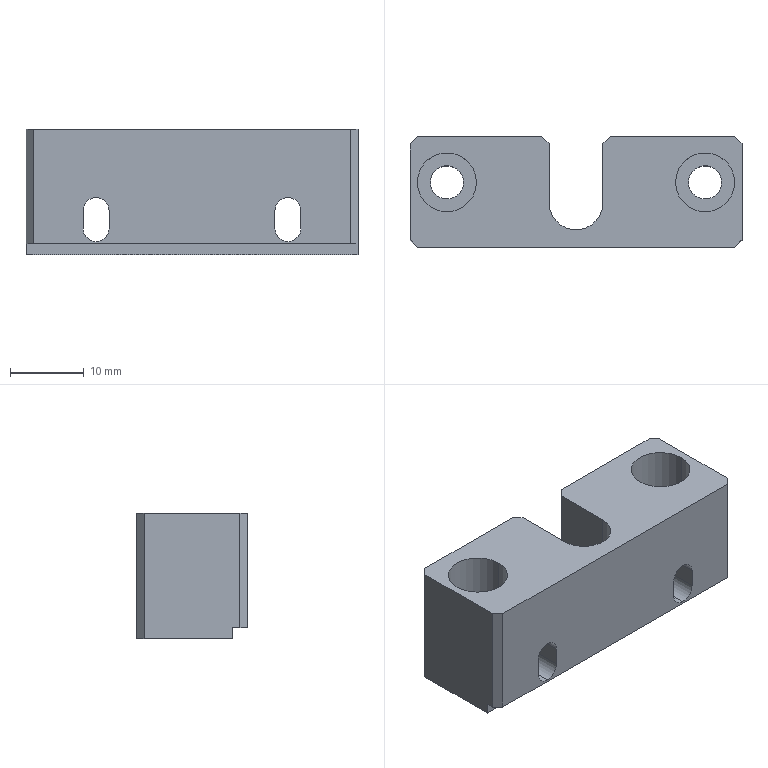Part | SolidWorks | features BaseBody 1 | 1 solid | 46 faces | box 45 x 15 x 17 mm | volume 8178 mm3 | plane 23 | cylinder 19 | cone 4 | commonest cylinder face diameters 3.5 x6 4 x4 4.5 x4 8 x4 7.3 x1
STEP:
#1=CARTESIAN_POINT('',(35.5,15.,-2.25));
#2=VERTEX_POINT('',#1);
#3=CARTESIAN_POINT('',(37.25,15.,-0.5));
#4=VERTEX_POINT('',#3);
#5=CARTESIAN_POINT('',(35.5,15.,-0.5));
#6=DIRECTION('',(0.,-1.,0.));
#7=DIRECTION('',(0.,0.,-1.));
#8=AXIS2_PLACEMENT_3D('',#5,#6,#7);
#9=CIRCLE('',#8,1.75);
#10=EDGE_CURVE('',#2,#4,#9,.T.);
#11=ORIENTED_EDGE('',*,*,#10,.F.);
#12=CARTESIAN_POINT('',(35.5,0.,-2.25));
#13=VERTEX_POINT('',#12);
#14=CARTESIAN_POINT('',(35.5,15.,-2.25));
#15=DIRECTION('',(0.,-1.,0.));
#16=VECTOR('',#15,1000.);
#17=LINE('',#14,#16);
#18=EDGE_CURVE('',#2,#13,#17,.T.);
#19=ORIENTED_EDGE('',*,*,#18,.T.);
#20=CARTESIAN_POINT('',(37.25,0.,-0.5));
#21=VERTEX_POINT('',#20);
#22=CARTESIAN_POINT('',(35.5,0.,-0.5));
#23=DIRECTION('',(0.,1.,0.));
#24=DIRECTION('',(0.,0.,-1.));
#25=AXIS2_PLACEMENT_3D('',#22,#23,#24);
#26=CIRCLE('',#25,1.75);
#27=EDGE_CURVE('',#21,#13,#26,.T.);
#28=ORIENTED_EDGE('',*,*,#27,.F.);
#29=CARTESIAN_POINT('',(37.25,15.,-0.5));
#30=DIRECTION('',(0.,-1.,0.));
#31=VECTOR('',#30,1000.);
#32=LINE('',#29,#31);
#33=EDGE_CURVE('',#4,#21,#32,.T.);
#34=ORIENTED_EDGE('',*,*,#33,.F.);
#35=EDGE_LOOP('',(#11,#19,#28,#34));
#36=FACE_OUTER_BOUND('',#35,.T.);
#37=CARTESIAN_POINT('',(35.5,15.,-0.5));
#38=DIRECTION('',(0.,-1.,0.));
#39=DIRECTION('',(0.,0.,-1.));
#40=AXIS2_PLACEMENT_3D('',#37,#38,#39);
#41=CYLINDRICAL_SURFACE('',#40,1.75);
#42=ADVANCED_FACE('',(#36),#41,.F.);
#43=CARTESIAN_POINT('',(9.5,15.,-2.25));
#44=VERTEX_POINT('',#43);
#45=CARTESIAN_POINT('',(11.25,15.,-0.5));
#46=VERTEX_POINT('',#45);
#47=CARTESIAN_POINT('',(9.5,15.,-0.5));
#48=DIRECTION('',(0.,-1.,0.));
#49=DIRECTION('',(0.,0.,-1.));
#50=AXIS2_PLACEMENT_3D('',#47,#48,#49);
#51=CIRCLE('',#50,1.75);
#52=EDGE_CURVE('',#44,#46,#51,.T.);
#53=ORIENTED_EDGE('',*,*,#52,.F.);
#54=CARTESIAN_POINT('',(9.5,0.,-2.25));
#55=VERTEX_POINT('',#54);
#56=CARTESIAN_POINT('',(9.5,15.,-2.25));
#57=DIRECTION('',(0.,-1.,0.));
#58=VECTOR('',#57,1000.);
#59=LINE('',#56,#58);
#60=EDGE_CURVE('',#44,#55,#59,.T.);
#61=ORIENTED_EDGE('',*,*,#60,.T.);
#62=CARTESIAN_POINT('',(11.25,0.,-0.5));
#63=VERTEX_POINT('',#62);
#64=CARTESIAN_POINT('',(9.5,0.,-0.5));
#65=DIRECTION('',(0.,1.,0.));
#66=DIRECTION('',(0.,0.,-1.));
#67=AXIS2_PLACEMENT_3D('',#64,#65,#66);
#68=CIRCLE('',#67,1.75);
#69=EDGE_CURVE('',#63,#55,#68,.T.);
#70=ORIENTED_EDGE('',*,*,#69,.F.);
#71=CARTESIAN_POINT('',(11.25,15.,-0.5));
#72=DIRECTION('',(0.,-1.,0.));
#73=VECTOR('',#72,1000.);
#74=LINE('',#71,#73);
#75=EDGE_CURVE('',#46,#63,#74,.T.);
#76=ORIENTED_EDGE('',*,*,#75,.F.);
#77=EDGE_LOOP('',(#53,#61,#70,#76));
#78=FACE_OUTER_BOUND('',#77,.T.);
#79=CARTESIAN_POINT('',(9.5,15.,-0.5));
#80=DIRECTION('',(0.,-1.,0.));
#81=DIRECTION('',(0.,0.,-1.));
#82=AXIS2_PLACEMENT_3D('',#79,#80,#81);
#83=CYLINDRICAL_SURFACE('',#82,1.75);
#84=ADVANCED_FACE('',(#78),#83,.F.);
#85=CARTESIAN_POINT('',(36.,8.8,7.));
#86=VERTEX_POINT('',#85);
#87=CARTESIAN_POINT('',(44.,8.8,7.));
#88=VERTEX_POINT('',#87);
#89=CARTESIAN_POINT('',(40.,8.8,7.));
#90=DIRECTION('',(0.,0.,1.));
#91=DIRECTION('',(1.,0.,0.));
#92=AXIS2_PLACEMENT_3D('',#89,#90,#91);
#93=CIRCLE('',#92,4.);
#94=EDGE_CURVE('',#86,#88,#93,.T.);
#95=ORIENTED_EDGE('',*,*,#94,.F.);
#96=CARTESIAN_POINT('',(36.,8.8,13.));
#97=VERTEX_POINT('',#96);
#98=CARTESIAN_POINT('',(36.,8.8,13.));
#99=DIRECTION('',(0.,0.,1.));
#100=VECTOR('',#99,1000.);
#101=LINE('',#98,#100);
#102=EDGE_CURVE('',#86,#97,#101,.T.);
#103=ORIENTED_EDGE('',*,*,#102,.T.);
#104=CARTESIAN_POINT('',(44.,8.8,13.));
#105=VERTEX_POINT('',#104);
#106=CARTESIAN_POINT('',(40.,8.8,13.));
#107=DIRECTION('',(0.,0.,-1.));
#108=DIRECTION('',(1.,0.,0.));
#109=AXIS2_PLACEMENT_3D('',#106,#107,#108);
#110=CIRCLE('',#109,4.);
#111=EDGE_CURVE('',#105,#97,#110,.T.);
#112=ORIENTED_EDGE('',*,*,#111,.F.);
#113=CARTESIAN_POINT('',(44.,8.8,13.));
#114=DIRECTION('',(0.,0.,1.));
#115=VECTOR('',#114,1000.);
#116=LINE('',#113,#115);
#117=EDGE_CURVE('',#88,#105,#116,.T.);
#118=ORIENTED_EDGE('',*,*,#117,.F.);
#119=EDGE_LOOP('',(#95,#103,#112,#118));
#120=FACE_OUTER_BOUND('',#119,.T.);
#121=CARTESIAN_POINT('',(40.,8.8,13.));
#122=DIRECTION('',(0.,0.,1.));
#123=DIRECTION('',(1.,0.,0.));
#124=AXIS2_PLACEMENT_3D('',#121,#122,#123);
#125=CYLINDRICAL_SURFACE('',#124,4.);
#126=ADVANCED_FACE('',(#120),#125,.F.);
#127=CARTESIAN_POINT('',(1.,8.8,7.));
#128=VERTEX_POINT('',#127);
#129=CARTESIAN_POINT('',(9.,8.8,7.));
#130=VERTEX_POINT('',#129);
#131=CARTESIAN_POINT('',(5.,8.8,7.));
#132=DIRECTION('',(0.,0.,1.));
#133=DIRECTION('',(1.,0.,0.));
#134=AXIS2_PLACEMENT_3D('',#131,#132,#133);
#135=CIRCLE('',#134,4.);
#136=EDGE_CURVE('',#128,#130,#135,.T.);
#137=ORIENTED_EDGE('',*,*,#136,.F.);
#138=CARTESIAN_POINT('',(1.,8.8,13.));
#139=VERTEX_POINT('',#138);
#140=CARTESIAN_POINT('',(1.,8.8,13.));
#141=DIRECTION('',(0.,0.,1.));
#142=VECTOR('',#141,1000.);
#143=LINE('',#140,#142);
#144=EDGE_CURVE('',#128,#139,#143,.T.);
#145=ORIENTED_EDGE('',*,*,#144,.T.);
#146=CARTESIAN_POINT('',(9.,8.8,13.));
#147=VERTEX_POINT('',#146);
#148=CARTESIAN_POINT('',(5.,8.8,13.));
#149=DIRECTION('',(0.,0.,-1.));
#150=DIRECTION('',(1.,0.,0.));
#151=AXIS2_PLACEMENT_3D('',#148,#149,#150);
#152=CIRCLE('',#151,4.);
#153=EDGE_CURVE('',#147,#139,#152,.T.);
#154=ORIENTED_EDGE('',*,*,#153,.F.);
#155=CARTESIAN_POINT('',(9.,8.8,13.));
#156=DIRECTION('',(0.,0.,1.));
#157=VECTOR('',#156,1000.);
#158=LINE('',#155,#157);
#159=EDGE_CURVE('',#130,#147,#158,.T.);
#160=ORIENTED_EDGE('',*,*,#159,.F.);
#161=EDGE_LOOP('',(#137,#145,#154,#160));
#162=FACE_OUTER_BOUND('',#161,.T.);
#163=CARTESIAN_POINT('',(5.,8.8,13.));
#164=DIRECTION('',(0.,0.,1.));
#165=DIRECTION('',(1.,0.,0.));
#166=AXIS2_PLACEMENT_3D('',#163,#164,#165);
#167=CYLINDRICAL_SURFACE('',#166,4.);
#168=ADVANCED_FACE('',(#162),#167,.F.);
#169=CARTESIAN_POINT('',(37.75,8.8,-4.));
#170=VERTEX_POINT('',#169);
#171=CARTESIAN_POINT('',(42.25,8.8,-4.));
#172=VERTEX_POINT('',#171);
#173=CARTESIAN_POINT('',(40.,8.8,-4.));
#174=DIRECTION('',(0.,0.,1.));
#175=DIRECTION('',(1.,0.,0.));
#176=AXIS2_PLACEMENT_3D('',#173,#174,#175);
#177=CIRCLE('',#176,2.25);
#178=EDGE_CURVE('',#170,#172,#177,.T.);
#179=ORIENTED_EDGE('',*,*,#178,.F.);
#180=CARTESIAN_POINT('',(37.75,8.8,7.));
#181=VERTEX_POINT('',#180);
#182=CARTESIAN_POINT('',(37.75,8.8,13.));
#183=DIRECTION('',(0.,0.,1.));
#184=VECTOR('',#183,1000.);
#185=LINE('',#182,#184);
#186=EDGE_CURVE('',#170,#181,#185,.T.);
#187=ORIENTED_EDGE('',*,*,#186,.T.);
#188=CARTESIAN_POINT('',(42.25,8.8,7.));
#189=VERTEX_POINT('',#188);
#190=CARTESIAN_POINT('',(40.,8.8,7.));
#191=DIRECTION('',(0.,0.,1.));
#192=DIRECTION('',(1.,0.,0.));
#193=AXIS2_PLACEMENT_3D('',#190,#191,#192);
#194=CIRCLE('',#193,2.25);
#195=EDGE_CURVE('',#181,#189,#194,.T.);
#196=ORIENTED_EDGE('',*,*,#195,.T.);
#197=CARTESIAN_POINT('',(42.25,8.8,13.));
#198=DIRECTION('',(0.,0.,1.));
#199=VECTOR('',#198,1000.);
#200=LINE('',#197,#199);
#201=EDGE_CURVE('',#172,#189,#200,.T.);
#202=ORIENTED_EDGE('',*,*,#201,.F.);
#203=EDGE_LOOP('',(#179,#187,#196,#202));
#204=FACE_OUTER_BOUND('',#203,.T.);
#205=CARTESIAN_POINT('',(40.,8.8,13.));
#206=DIRECTION('',(0.,0.,1.));
#207=DIRECTION('',(1.,0.,0.));
#208=AXIS2_PLACEMENT_3D('',#205,#206,#207);
#209=CYLINDRICAL_SURFACE('',#208,2.25);
#210=ADVANCED_FACE('',(#204),#209,.F.);
#211=CARTESIAN_POINT('',(2.75,8.8,-4.));
#212=VERTEX_POINT('',#211);
#213=CARTESIAN_POINT('',(7.25,8.8,-4.));
#214=VERTEX_POINT('',#213);
#215=CARTESIAN_POINT('',(5.,8.8,-4.));
#216=DIRECTION('',(0.,0.,1.));
#217=DIRECTION('',(1.,0.,0.));
#218=AXIS2_PLACEMENT_3D('',#215,#216,#217);
#219=CIRCLE('',#218,2.25);
#220=EDGE_CURVE('',#212,#214,#219,.T.);
#221=ORIENTED_EDGE('',*,*,#220,.F.);
#222=CARTESIAN_POINT('',(2.75,8.8,7.));
#223=VERTEX_POINT('',#222);
#224=CARTESIAN_POINT('',(2.75,8.8,13.));
#225=DIRECTION('',(0.,0.,1.));
#226=VECTOR('',#225,1000.);
#227=LINE('',#224,#226);
#228=EDGE_CURVE('',#212,#223,#227,.T.);
#229=ORIENTED_EDGE('',*,*,#228,.T.);
#230=CARTESIAN_POINT('',(7.25,8.8,7.));
#231=VERTEX_POINT('',#230);
#232=CARTESIAN_POINT('',(5.,8.8,7.));
#233=DIRECTION('',(0.,0.,1.));
#234=DIRECTION('',(1.,0.,0.));
#235=AXIS2_PLACEMENT_3D('',#232,#233,#234);
#236=CIRCLE('',#235,2.25);
#237=EDGE_CURVE('',#223,#231,#236,.T.);
#238=ORIENTED_EDGE('',*,*,#237,.T.);
#239=CARTESIAN_POINT('',(7.25,8.8,13.));
#240=DIRECTION('',(0.,0.,1.));
#241=VECTOR('',#240,1000.);
#242=LINE('',#239,#241);
#243=EDGE_CURVE('',#214,#231,#242,.T.);
#244=ORIENTED_EDGE('',*,*,#243,.F.);
#245=EDGE_LOOP('',(#221,#229,#238,#244));
#246=FACE_OUTER_BOUND('',#245,.T.);
#247=CARTESIAN_POINT('',(5.,8.8,13.));
#248=DIRECTION('',(0.,0.,1.));
#249=DIRECTION('',(1.,0.,0.));
#250=AXIS2_PLACEMENT_3D('',#247,#248,#249);
#251=CYLINDRICAL_SURFACE('',#250,2.25);
#252=ADVANCED_FACE('',(#246),#251,.F.);
#253=CARTESIAN_POINT('',(15.5,8.8,1.));
#254=VERTEX_POINT('',#253);
#255=CARTESIAN_POINT('',(11.5,8.8,1.));
#256=VERTEX_POINT('',#255);
#257=CARTESIAN_POINT('',(13.5,8.8,1.));
#258=DIRECTION('',(0.,0.,-1.));
#259=DIRECTION('',(-1.,0.,0.));
#260=AXIS2_PLACEMENT_3D('',#257,#258,#259);
#261=CIRCLE('',#260,2.);
#262=EDGE_CURVE('',#254,#256,#261,.T.);
#263=ORIENTED_EDGE('',*,*,#262,.F.);
#264=CARTESIAN_POINT('',(15.5,8.8,-4.));
#265=VERTEX_POINT('',#264);
#266=CARTESIAN_POINT('',(15.5,8.8,-4.));
#267=DIRECTION('',(0.,0.,-1.));
#268=VECTOR('',#267,1000.);
#269=LINE('',#266,#268);
#270=EDGE_CURVE('',#254,#265,#269,.T.);
#271=ORIENTED_EDGE('',*,*,#270,.T.);
#272=CARTESIAN_POINT('',(11.5,8.8,-4.));
#273=VERTEX_POINT('',#272);
#274=CARTESIAN_POINT('',(13.5,8.8,-4.));
#275=DIRECTION('',(0.,0.,1.));
#276=DIRECTION('',(-1.,0.,0.));
#277=AXIS2_PLACEMENT_3D('',#274,#275,#276);
#278=CIRCLE('',#277,2.);
#279=EDGE_CURVE('',#273,#265,#278,.T.);
#280=ORIENTED_EDGE('',*,*,#279,.F.);
#281=CARTESIAN_POINT('',(11.5,8.8,-4.));
#282=DIRECTION('',(0.,0.,-1.));
#283=VECTOR('',#282,1000.);
#284=LINE('',#281,#283);
#285=EDGE_CURVE('',#256,#273,#284,.T.);
#286=ORIENTED_EDGE('',*,*,#285,.F.);
#287=EDGE_LOOP('',(#263,#271,#280,#286));
#288=FACE_OUTER_BOUND('',#287,.T.);
#289=CARTESIAN_POINT('',(13.5,8.8,-4.));
#290=DIRECTION('',(0.,0.,-1.));
#291=DIRECTION('',(-1.,0.,0.));
#292=AXIS2_PLACEMENT_3D('',#289,#290,#291);
#293=CYLINDRICAL_SURFACE('',#292,2.);
#294=ADVANCED_FACE('',(#288),#293,.F.);
#295=CARTESIAN_POINT('',(33.5,8.8,1.));
#296=VERTEX_POINT('',#295);
#297=CARTESIAN_POINT('',(29.5,8.8,1.));
#298=VERTEX_POINT('',#297);
#299=CARTESIAN_POINT('',(31.5,8.8,1.));
#300=DIRECTION('',(0.,0.,-1.));
#301=DIRECTION('',(-1.,0.,0.));
#302=AXIS2_PLACEMENT_3D('',#299,#300,#301);
#303=CIRCLE('',#302,2.);
#304=EDGE_CURVE('',#296,#298,#303,.T.);
#305=ORIENTED_EDGE('',*,*,#304,.F.);
#306=CARTESIAN_POINT('',(33.5,8.8,-4.));
#307=VERTEX_POINT('',#306);
#308=CARTESIAN_POINT('',(33.5,8.8,-4.));
#309=DIRECTION('',(0.,0.,-1.));
#310=VECTOR('',#309,1000.);
#311=LINE('',#308,#310);
#312=EDGE_CURVE('',#296,#307,#311,.T.);
#313=ORIENTED_EDGE('',*,*,#312,.T.);
#314=CARTESIAN_POINT('',(29.5,8.8,-4.));
#315=VERTEX_POINT('',#314);
#316=CARTESIAN_POINT('',(31.5,8.8,-4.));
#317=DIRECTION('',(0.,0.,1.));
#318=DIRECTION('',(-1.,0.,0.));
#319=AXIS2_PLACEMENT_3D('',#316,#317,#318);
#320=CIRCLE('',#319,2.);
#321=EDGE_CURVE('',#315,#307,#320,.T.);
#322=ORIENTED_EDGE('',*,*,#321,.F.);
#323=CARTESIAN_POINT('',(29.5,8.8,-4.));
#324=DIRECTION('',(0.,0.,-1.));
#325=VECTOR('',#324,1000.);
#326=LINE('',#323,#325);
#327=EDGE_CURVE('',#298,#315,#326,.T.);
#328=ORIENTED_EDGE('',*,*,#327,.F.);
#329=EDGE_LOOP('',(#305,#313,#322,#328));
#330=FACE_OUTER_BOUND('',#329,.T.);
#331=CARTESIAN_POINT('',(31.5,8.8,-4.));
#332=DIRECTION('',(0.,0.,-1.));
#333=DIRECTION('',(-1.,0.,0.));
#334=AXIS2_PLACEMENT_3D('',#331,#332,#333);
#335=CYLINDRICAL_SURFACE('',#334,2.);
#336=ADVANCED_FACE('',(#330),#335,.F.);
#337=CARTESIAN_POINT('',(13.5,8.8,2.202));
#338=VERTEX_POINT('',#337);
#339=CARTESIAN_POINT('',(11.5,8.8,1.));
#340=DIRECTION('',(-0.8572,0.,-0.515));
#341=VECTOR('',#340,1000.);
#342=LINE('',#339,#341);
#343=EDGE_CURVE('',#338,#256,#342,.T.);
#344=ORIENTED_EDGE('',*,*,#343,.F.);
#345=CARTESIAN_POINT('',(15.5,8.8,1.));
#346=DIRECTION('',(0.8572,0.,-0.515));
#347=VECTOR('',#346,1000.);
#348=LINE('',#345,#347);
#349=EDGE_CURVE('',#338,#254,#348,.T.);
#350=ORIENTED_EDGE('',*,*,#349,.T.);
#351=ORIENTED_EDGE('',*,*,#262,.T.);
#352=EDGE_LOOP('',(#344,#350,#351));
#353=FACE_OUTER_BOUND('',#352,.T.);
#354=CARTESIAN_POINT('',(13.5,8.8,1.));
#355=DIRECTION('',(0.,0.,-1.));
#356=DIRECTION('',(-1.,0.,0.));
#357=AXIS2_PLACEMENT_3D('',#354,#355,#356);
#358=CONICAL_SURFACE('',#357,2.,1.03);
#359=ADVANCED_FACE('',(#353),#358,.F.);
#360=CARTESIAN_POINT('',(31.5,8.8,2.202));
#361=VERTEX_POINT('',#360);
#362=CARTESIAN_POINT('',(29.5,8.8,1.));
#363=DIRECTION('',(-0.8572,0.,-0.515));
#364=VECTOR('',#363,1000.);
#365=LINE('',#362,#364);
#366=EDGE_CURVE('',#361,#298,#365,.T.);
#367=ORIENTED_EDGE('',*,*,#366,.F.);
#368=CARTESIAN_POINT('',(33.5,8.8,1.));
#369=DIRECTION('',(0.8572,0.,-0.515));
#370=VECTOR('',#369,1000.);
#371=LINE('',#368,#370);
#372=EDGE_CURVE('',#361,#296,#371,.T.);
#373=ORIENTED_EDGE('',*,*,#372,.T.);
#374=ORIENTED_EDGE('',*,*,#304,.T.);
#375=EDGE_LOOP('',(#367,#373,#374));
#376=FACE_OUTER_BOUND('',#375,.T.);
#377=CARTESIAN_POINT('',(31.5,8.8,1.));
#378=DIRECTION('',(0.,0.,-1.));
#379=DIRECTION('',(-1.,0.,0.));
#380=AXIS2_PLACEMENT_3D('',#377,#378,#379);
#381=CONICAL_SURFACE('',#380,2.,1.03);
#382=ADVANCED_FACE('',(#376),#381,.F.);
#383=ORIENTED_EDGE('',*,*,#27,.T.);
#384=CARTESIAN_POINT('',(33.75,0.,-0.5));
#385=VERTEX_POINT('',#384);
#386=CARTESIAN_POINT('',(35.5,0.,-0.5));
#387=DIRECTION('',(0.,1.,0.));
#388=DIRECTION('',(0.,0.,-1.));
#389=AXIS2_PLACEMENT_3D('',#386,#387,#388);
#390=CIRCLE('',#389,1.75);
#391=EDGE_CURVE('',#13,#385,#390,.T.);
#392=ORIENTED_EDGE('',*,*,#391,.T.);
#393=CARTESIAN_POINT('',(33.75,0.,2.));
#394=VERTEX_POINT('',#393);
#395=CARTESIAN_POINT('',(33.75,0.,0.));
#396=DIRECTION('',(0.,0.,1.));
#397=VECTOR('',#396,1000.);
#398=LINE('',#395,#397);
#399=EDGE_CURVE('',#385,#394,#398,.T.);
#400=ORIENTED_EDGE('',*,*,#399,.T.);
#401=CARTESIAN_POINT('',(37.25,0.,2.));
#402=VERTEX_POINT('',#401);
#403=CARTESIAN_POINT('',(35.5,0.,2.));
#404=DIRECTION('',(0.,1.,0.));
#405=DIRECTION('',(0.,0.,-1.));
#406=AXIS2_PLACEMENT_3D('',#403,#404,#405);
#407=CIRCLE('',#406,1.75);
#408=EDGE_CURVE('',#394,#402,#407,.T.);
#409=ORIENTED_EDGE('',*,*,#408,.T.);
#410=CARTESIAN_POINT('',(37.25,0.,0.));
#411=DIRECTION('',(0.,0.,-1.));
#412=VECTOR('',#411,1000.);
#413=LINE('',#410,#412);
#414=EDGE_CURVE('',#402,#21,#413,.T.);
#415=ORIENTED_EDGE('',*,*,#414,.T.);
#416=EDGE_LOOP('',(#383,#392,#400,#409,#415));
#417=FACE_BOUND('',#416,.T.);
#418=CARTESIAN_POINT('',(11.25,0.,2.));
#419=VERTEX_POINT('',#418);
#420=CARTESIAN_POINT('',(11.25,0.,0.));
#421=DIRECTION('',(0.,0.,-1.));
#422=VECTOR('',#421,1000.);
#423=LINE('',#420,#422);
#424=EDGE_CURVE('',#419,#63,#423,.T.);
#425=ORIENTED_EDGE('',*,*,#424,.T.);
#426=ORIENTED_EDGE('',*,*,#69,.T.);
#427=CARTESIAN_POINT('',(7.75,0.,-0.5));
#428=VERTEX_POINT('',#427);
#429=CARTESIAN_POINT('',(9.5,0.,-0.5));
#430=DIRECTION('',(0.,1.,0.));
#431=DIRECTION('',(0.,0.,-1.));
#432=AXIS2_PLACEMENT_3D('',#429,#430,#431);
#433=CIRCLE('',#432,1.75);
#434=EDGE_CURVE('',#55,#428,#433,.T.);
#435=ORIENTED_EDGE('',*,*,#434,.T.);
#436=CARTESIAN_POINT('',(7.75,0.,2.));
#437=VERTEX_POINT('',#436);
#438=CARTESIAN_POINT('',(7.75,0.,0.));
#439=DIRECTION('',(0.,0.,1.));
#440=VECTOR('',#439,1000.);
#441=LINE('',#438,#440);
#442=EDGE_CURVE('',#428,#437,#441,.T.);
#443=ORIENTED_EDGE('',*,*,#442,.T.);
#444=CARTESIAN_POINT('',(9.5,0.,2.));
#445=DIRECTION('',(0.,1.,0.));
#446=DIRECTION('',(0.,0.,-1.));
#447=AXIS2_PLACEMENT_3D('',#444,#445,#446);
#448=CIRCLE('',#447,1.75);
#449=EDGE_CURVE('',#437,#419,#448,.T.);
#450=ORIENTED_EDGE('',*,*,#449,.T.);
#451=EDGE_LOOP('',(#425,#426,#435,#443,#450));
#452=FACE_BOUND('',#451,.T.);
#453=CARTESIAN_POINT('',(1.,0.,-2.5));
#454=VERTEX_POINT('',#453);
#455=CARTESIAN_POINT('',(44.,0.,-2.5));
#456=VERTEX_POINT('',#455);
#457=CARTESIAN_POINT('',(0.,0.,-2.5));
#458=DIRECTION('',(1.,0.,0.));
#459=VECTOR('',#458,1000.);
#460=LINE('',#457,#459);
#461=EDGE_CURVE('',#454,#456,#460,.T.);
#462=ORIENTED_EDGE('',*,*,#461,.T.);
#463=CARTESIAN_POINT('',(44.,0.,13.));
#464=VERTEX_POINT('',#463);
#465=CARTESIAN_POINT('',(44.,0.,0.));
#466=DIRECTION('',(0.,0.,1.));
#467=VECTOR('',#466,1000.);
#468=LINE('',#465,#467);
#469=EDGE_CURVE('',#456,#464,#468,.T.);
#470=ORIENTED_EDGE('',*,*,#469,.T.);
#471=CARTESIAN_POINT('',(1.,0.,13.));
#472=VERTEX_POINT('',#471);
#473=CARTESIAN_POINT('',(0.,0.,13.));
#474=DIRECTION('',(-1.,0.,0.));
#475=VECTOR('',#474,1000.);
#476=LINE('',#473,#475);
#477=EDGE_CURVE('',#464,#472,#476,.T.);
#478=ORIENTED_EDGE('',*,*,#477,.T.);
#479=CARTESIAN_POINT('',(1.,0.,0.));
#480=DIRECTION('',(0.,0.,-1.));
#481=VECTOR('',#480,1000.);
#482=LINE('',#479,#481);
#483=EDGE_CURVE('',#472,#454,#482,.T.);
#484=ORIENTED_EDGE('',*,*,#483,.T.);
#485=EDGE_LOOP('',(#462,#470,#478,#484));
#486=FACE_OUTER_BOUND('',#485,.T.);
#487=CARTESIAN_POINT('',(0.,0.,0.));
#488=DIRECTION('',(0.,-1.,0.));
#489=DIRECTION('',(0.,0.,-1.));
#490=AXIS2_PLACEMENT_3D('',#487,#488,#489);
#491=PLANE('',#490);
#492=ADVANCED_FACE('',(#417,#452,#486),#491,.T.);
#493=CARTESIAN_POINT('',(33.75,15.,-0.5));
#494=VERTEX_POINT('',#493);
#495=CARTESIAN_POINT('',(33.75,15.,-0.5));
#496=DIRECTION('',(0.,-1.,0.));
#497=VECTOR('',#496,1000.);
#498=LINE('',#495,#497);
#499=EDGE_CURVE('',#494,#385,#498,.T.);
#500=ORIENTED_EDGE('',*,*,#499,.F.);
#501=CARTESIAN_POINT('',(33.75,15.,2.));
#502=VERTEX_POINT('',#501);
#503=CARTESIAN_POINT('',(33.75,15.,2.));
#504=DIRECTION('',(0.,0.,-1.));
#505=VECTOR('',#504,1000.);
#506=LINE('',#503,#505);
#507=EDGE_CURVE('',#502,#494,#506,.T.);
#508=ORIENTED_EDGE('',*,*,#507,.F.);
#509=CARTESIAN_POINT('',(33.75,15.,2.));
#510=DIRECTION('',(0.,1.,0.));
#511=VECTOR('',#510,1000.);
#512=LINE('',#509,#511);
#513=EDGE_CURVE('',#394,#502,#512,.T.);
#514=ORIENTED_EDGE('',*,*,#513,.F.);
#515=ORIENTED_EDGE('',*,*,#399,.F.);
#516=EDGE_LOOP('',(#500,#508,#514,#515));
#517=FACE_OUTER_BOUND('',#516,.T.);
#518=CARTESIAN_POINT('',(33.75,15.,2.));
#519=DIRECTION('',(-1.,0.,0.));
#520=DIRECTION('',(0.,0.,1.));
#521=AXIS2_PLACEMENT_3D('',#518,#519,#520);
#522=PLANE('',#521);
#523=ADVANCED_FACE('',(#517),#522,.F.);
#524=ORIENTED_EDGE('',*,*,#18,.F.);
#525=CARTESIAN_POINT('',(35.5,15.,-0.5));
#526=DIRECTION('',(0.,-1.,0.));
#527=DIRECTION('',(0.,0.,-1.));
#528=AXIS2_PLACEMENT_3D('',#525,#526,#527);
#529=CIRCLE('',#528,1.75);
#530=EDGE_CURVE('',#494,#2,#529,.T.);
#531=ORIENTED_EDGE('',*,*,#530,.F.);
#532=ORIENTED_EDGE('',*,*,#499,.T.);
#533=ORIENTED_EDGE('',*,*,#391,.F.);
#534=EDGE_LOOP('',(#524,#531,#532,#533));
#535=FACE_OUTER_BOUND('',#534,.T.);
#536=CARTESIAN_POINT('',(35.5,15.,-0.5));
#537=DIRECTION('',(0.,-1.,0.));
#538=DIRECTION('',(0.,0.,-1.));
#539=AXIS2_PLACEMENT_3D('',#536,#537,#538);
#540=CYLINDRICAL_SURFACE('',#539,1.75);
#541=ADVANCED_FACE('',(#535),#540,.F.);
#542=CARTESIAN_POINT('',(37.25,15.,2.));
#543=VERTEX_POINT('',#542);
#544=CARTESIAN_POINT('',(37.25,15.,2.));
#545=DIRECTION('',(0.,-1.,0.));
#546=VECTOR('',#545,1000.);
#547=LINE('',#544,#546);
#548=EDGE_CURVE('',#543,#402,#547,.T.);
#549=ORIENTED_EDGE('',*,*,#548,.F.);
#550=CARTESIAN_POINT('',(37.25,15.,-0.5));
#551=DIRECTION('',(0.,0.,1.));
#552=VECTOR('',#551,1000.);
#553=LINE('',#550,#552);
#554=EDGE_CURVE('',#4,#543,#553,.T.);
#555=ORIENTED_EDGE('',*,*,#554,.F.);
#556=ORIENTED_EDGE('',*,*,#33,.T.);
#557=ORIENTED_EDGE('',*,*,#414,.F.);
#558=EDGE_LOOP('',(#549,#555,#556,#557));
#559=FACE_OUTER_BOUND('',#558,.T.);
#560=CARTESIAN_POINT('',(37.25,15.,-0.5));
#561=DIRECTION('',(1.,0.,0.));
#562=DIRECTION('',(0.,0.,-1.));
#563=AXIS2_PLACEMENT_3D('',#560,#561,#562);
#564=PLANE('',#563);
#565=ADVANCED_FACE('',(#559),#564,.F.);
#566=ORIENTED_EDGE('',*,*,#513,.T.);
#567=CARTESIAN_POINT('',(35.5,15.,2.));
#568=DIRECTION('',(0.,-1.,0.));
#569=DIRECTION('',(0.,0.,-1.));
#570=AXIS2_PLACEMENT_3D('',#567,#568,#569);
#571=CIRCLE('',#570,1.75);
#572=EDGE_CURVE('',#543,#502,#571,.T.);
#573=ORIENTED_EDGE('',*,*,#572,.F.);
#574=ORIENTED_EDGE('',*,*,#548,.T.);
#575=ORIENTED_EDGE('',*,*,#408,.F.);
#576=EDGE_LOOP('',(#566,#573,#574,#575));
#577=FACE_OUTER_BOUND('',#576,.T.);
#578=CARTESIAN_POINT('',(35.5,15.,2.));
#579=DIRECTION('',(0.,-1.,0.));
#580=DIRECTION('',(0.,0.,-1.));
#581=AXIS2_PLACEMENT_3D('',#578,#579,#580);
#582=CYLINDRICAL_SURFACE('',#581,1.75);
#583=ADVANCED_FACE('',(#577),#582,.F.);
#584=ORIENTED_EDGE('',*,*,#60,.F.);
#585=CARTESIAN_POINT('',(7.75,15.,-0.5));
#586=VERTEX_POINT('',#585);
#587=CARTESIAN_POINT('',(9.5,15.,-0.5));
#588=DIRECTION('',(0.,-1.,0.));
#589=DIRECTION('',(0.,0.,-1.));
#590=AXIS2_PLACEMENT_3D('',#587,#588,#589);
#591=CIRCLE('',#590,1.75);
#592=EDGE_CURVE('',#586,#44,#591,.T.);
#593=ORIENTED_EDGE('',*,*,#592,.F.);
#594=CARTESIAN_POINT('',(7.75,15.,-0.5));
#595=DIRECTION('',(0.,-1.,0.));
#596=VECTOR('',#595,1000.);
#597=LINE('',#594,#596);
#598=EDGE_CURVE('',#586,#428,#597,.T.);
#599=ORIENTED_EDGE('',*,*,#598,.T.);
#600=ORIENTED_EDGE('',*,*,#434,.F.);
#601=EDGE_LOOP('',(#584,#593,#599,#600));
#602=FACE_OUTER_BOUND('',#601,.T.);
#603=CARTESIAN_POINT('',(9.5,15.,-0.5));
#604=DIRECTION('',(0.,-1.,0.));
#605=DIRECTION('',(0.,0.,-1.));
#606=AXIS2_PLACEMENT_3D('',#603,#604,#605);
#607=CYLINDRICAL_SURFACE('',#606,1.75);
#608=ADVANCED_FACE('',(#602),#607,.F.);
#609=CARTESIAN_POINT('',(11.25,15.,2.));
#610=VERTEX_POINT('',#609);
#611=CARTESIAN_POINT('',(11.25,15.,2.));
#612=DIRECTION('',(0.,-1.,0.));
#613=VECTOR('',#612,1000.);
#614=LINE('',#611,#613);
#615=EDGE_CURVE('',#610,#419,#614,.T.);
#616=ORIENTED_EDGE('',*,*,#615,.F.);
#617=CARTESIAN_POINT('',(11.25,15.,2.));
#618=DIRECTION('',(0.,0.,1.));
#619=VECTOR('',#618,1000.);
#620=LINE('',#617,#619);
#621=EDGE_CURVE('',#46,#610,#620,.T.);
#622=ORIENTED_EDGE('',*,*,#621,.F.);
#623=ORIENTED_EDGE('',*,*,#75,.T.);
#624=ORIENTED_EDGE('',*,*,#424,.F.);
#625=EDGE_LOOP('',(#616,#622,#623,#624));
#626=FACE_OUTER_BOUND('',#625,.T.);
#627=CARTESIAN_POINT('',(11.25,15.,2.));
#628=DIRECTION('',(1.,0.,0.));
#629=DIRECTION('',(0.,0.,-1.));
#630=AXIS2_PLACEMENT_3D('',#627,#628,#629);
#631=PLANE('',#630);
#632=ADVANCED_FACE('',(#626),#631,.F.);
#633=CARTESIAN_POINT('',(7.75,15.,2.));
#634=VERTEX_POINT('',#633);
#635=CARTESIAN_POINT('',(7.75,15.,2.));
#636=DIRECTION('',(0.,-1.,0.));
#637=VECTOR('',#636,1000.);
#638=LINE('',#635,#637);
#639=EDGE_CURVE('',#634,#437,#638,.T.);
#640=ORIENTED_EDGE('',*,*,#639,.F.);
#641=CARTESIAN_POINT('',(9.5,15.,2.));
#642=DIRECTION('',(0.,-1.,0.));
#643=DIRECTION('',(0.,0.,-1.));
#644=AXIS2_PLACEMENT_3D('',#641,#642,#643);
#645=CIRCLE('',#644,1.75);
#646=EDGE_CURVE('',#610,#634,#645,.T.);
#647=ORIENTED_EDGE('',*,*,#646,.F.);
#648=ORIENTED_EDGE('',*,*,#615,.T.);
#649=ORIENTED_EDGE('',*,*,#449,.F.);
#650=EDGE_LOOP('',(#640,#647,#648,#649));
#651=FACE_OUTER_BOUND('',#650,.T.);
#652=CARTESIAN_POINT('',(9.5,15.,2.));
#653=DIRECTION('',(0.,-1.,0.));
#654=DIRECTION('',(0.,0.,-1.));
#655=AXIS2_PLACEMENT_3D('',#652,#653,#654);
#656=CYLINDRICAL_SURFACE('',#655,1.75);
#657=ADVANCED_FACE('',(#651),#656,.F.);
#658=ORIENTED_EDGE('',*,*,#598,.F.);
#659=CARTESIAN_POINT('',(7.75,15.,-0.5));
#660=DIRECTION('',(0.,0.,-1.));
#661=VECTOR('',#660,1000.);
#662=LINE('',#659,#661);
#663=EDGE_CURVE('',#634,#586,#662,.T.);
#664=ORIENTED_EDGE('',*,*,#663,.F.);
#665=ORIENTED_EDGE('',*,*,#639,.T.);
#666=ORIENTED_EDGE('',*,*,#442,.F.);
#667=EDGE_LOOP('',(#658,#664,#665,#666));
#668=FACE_OUTER_BOUND('',#667,.T.);
#669=CARTESIAN_POINT('',(7.75,15.,-0.5));
#670=DIRECTION('',(-1.,0.,0.));
#671=DIRECTION('',(0.,0.,1.));
#672=AXIS2_PLACEMENT_3D('',#669,#670,#671);
#673=PLANE('',#672);
#674=ADVANCED_FACE('',(#668),#673,.F.);
#675=CARTESIAN_POINT('',(45.,1.,13.));
#676=VERTEX_POINT('',#675);
#677=CARTESIAN_POINT('',(45.,1.,-2.5));
#678=VERTEX_POINT('',#677);
#679=CARTESIAN_POINT('',(45.,1.,0.));
#680=DIRECTION('',(0.,0.,-1.));
#681=VECTOR('',#680,1000.);
#682=LINE('',#679,#681);
#683=EDGE_CURVE('',#676,#678,#682,.T.);
#684=ORIENTED_EDGE('',*,*,#683,.F.);
#685=CARTESIAN_POINT('',(44.,0.,13.));
#686=DIRECTION('',(0.7071,0.7071,0.));
#687=VECTOR('',#686,1000.);
#688=LINE('',#685,#687);
#689=EDGE_CURVE('',#464,#676,#688,.T.);
#690=ORIENTED_EDGE('',*,*,#689,.F.);
#691=ORIENTED_EDGE('',*,*,#469,.F.);
#692=CARTESIAN_POINT('',(44.,0.,-2.5));
#693=DIRECTION('',(-0.7071,-0.7071,0.));
#694=VECTOR('',#693,1000.);
#695=LINE('',#692,#694);
#696=EDGE_CURVE('',#678,#456,#695,.T.);
#697=ORIENTED_EDGE('',*,*,#696,.F.);
#698=EDGE_LOOP('',(#684,#690,#691,#697));
#699=FACE_OUTER_BOUND('',#698,.T.);
#700=CARTESIAN_POINT('',(44.,0.,0.));
#701=DIRECTION('',(-0.7071,0.7071,0.));
#702=DIRECTION('',(-0.7071,-0.7071,0.));
#703=AXIS2_PLACEMENT_3D('',#700,#701,#702);
#704=PLANE('',#703);
#705=ADVANCED_FACE('',(#699),#704,.F.);
#706=CARTESIAN_POINT('',(0.,1.,-2.5));
#707=VERTEX_POINT('',#706);
#708=CARTESIAN_POINT('',(0.,1.,-2.5));
#709=DIRECTION('',(0.7071,-0.7071,0.));
#710=VECTOR('',#709,1000.);
#711=LINE('',#708,#710);
#712=EDGE_CURVE('',#707,#454,#711,.T.);
#713=ORIENTED_EDGE('',*,*,#712,.F.);
#714=CARTESIAN_POINT('',(0.,2.,-2.5));
#715=VERTEX_POINT('',#714);
#716=CARTESIAN_POINT('',(0.,15.,-2.5));
#717=DIRECTION('',(0.,-1.,0.));
#718=VECTOR('',#717,1000.);
#719=LINE('',#716,#718);
#720=EDGE_CURVE('',#715,#707,#719,.T.);
#721=ORIENTED_EDGE('',*,*,#720,.F.);
#722=CARTESIAN_POINT('',(45.,2.,-2.5));
#723=VERTEX_POINT('',#722);
#724=CARTESIAN_POINT('',(0.,2.,-2.5));
#725=DIRECTION('',(-1.,0.,0.));
#726=VECTOR('',#725,1000.);
#727=LINE('',#724,#726);
#728=EDGE_CURVE('',#723,#715,#727,.T.);
#729=ORIENTED_EDGE('',*,*,#728,.F.);
#730=CARTESIAN_POINT('',(45.,0.,-2.5));
#731=DIRECTION('',(0.,1.,0.));
#732=VECTOR('',#731,1000.);
#733=LINE('',#730,#732);
#734=EDGE_CURVE('',#678,#723,#733,.T.);
#735=ORIENTED_EDGE('',*,*,#734,.F.);
#736=ORIENTED_EDGE('',*,*,#696,.T.);
#737=ORIENTED_EDGE('',*,*,#461,.F.);
#738=EDGE_LOOP('',(#713,#721,#729,#735,#736,#737));
#739=FACE_OUTER_BOUND('',#738,.T.);
#740=CARTESIAN_POINT('',(0.,0.,-2.5));
#741=DIRECTION('',(0.,0.,1.));
#742=DIRECTION('',(1.,0.,0.));
#743=AXIS2_PLACEMENT_3D('',#740,#741,#742);
#744=PLANE('',#743);
#745=ADVANCED_FACE('',(#739),#744,.F.);
#746=CARTESIAN_POINT('',(0.,1.,13.));
#747=VERTEX_POINT('',#746);
#748=CARTESIAN_POINT('',(0.,1.,0.));
#749=DIRECTION('',(0.,0.,1.));
#750=VECTOR('',#749,1000.);
#751=LINE('',#748,#750);
#752=EDGE_CURVE('',#707,#747,#751,.T.);
#753=ORIENTED_EDGE('',*,*,#752,.F.);
#754=ORIENTED_EDGE('',*,*,#712,.T.);
#755=ORIENTED_EDGE('',*,*,#483,.F.);
#756=CARTESIAN_POINT('',(1.,0.,13.));
#757=DIRECTION('',(0.7071,-0.7071,0.));
#758=VECTOR('',#757,1000.);
#759=LINE('',#756,#758);
#760=EDGE_CURVE('',#747,#472,#759,.T.);
#761=ORIENTED_EDGE('',*,*,#760,.F.);
#762=EDGE_LOOP('',(#753,#754,#755,#761));
#763=FACE_OUTER_BOUND('',#762,.T.);
#764=CARTESIAN_POINT('',(1.,0.,0.));
#765=DIRECTION('',(0.7071,0.7071,0.));
#766=DIRECTION('',(-0.7071,0.7071,0.));
#767=AXIS2_PLACEMENT_3D('',#764,#765,#766);
#768=PLANE('',#767);
#769=ADVANCED_FACE('',(#763),#768,.F.);
#770=ORIENTED_EDGE('',*,*,#111,.T.);
#771=CARTESIAN_POINT('',(40.,8.8,13.));
#772=DIRECTION('',(0.,0.,-1.));
#773=DIRECTION('',(1.,0.,0.));
#774=AXIS2_PLACEMENT_3D('',#771,#772,#773);
#775=CIRCLE('',#774,4.);
#776=EDGE_CURVE('',#97,#105,#775,.T.);
#777=ORIENTED_EDGE('',*,*,#776,.T.);
#778=EDGE_LOOP('',(#770,#777));
#779=FACE_BOUND('',#778,.T.);
#780=ORIENTED_EDGE('',*,*,#153,.T.);
#781=CARTESIAN_POINT('',(5.,8.8,13.));
#782=DIRECTION('',(0.,0.,-1.));
#783=DIRECTION('',(1.,0.,0.));
#784=AXIS2_PLACEMENT_3D('',#781,#782,#783);
#785=CIRCLE('',#784,4.);
#786=EDGE_CURVE('',#139,#147,#785,.T.);
#787=ORIENTED_EDGE('',*,*,#786,.T.);
#788=EDGE_LOOP('',(#780,#787));
#789=FACE_BOUND('',#788,.T.);
#790=CARTESIAN_POINT('',(26.15,14.,13.));
#791=VERTEX_POINT('',#790);
#792=CARTESIAN_POINT('',(26.15,6.,13.));
#793=VERTEX_POINT('',#792);
#794=CARTESIAN_POINT('',(26.15,15.,13.));
#795=DIRECTION('',(0.,-1.,0.));
#796=VECTOR('',#795,1000.);
#797=LINE('',#794,#796);
#798=EDGE_CURVE('',#791,#793,#797,.T.);
#799=ORIENTED_EDGE('',*,*,#798,.T.);
#800=CARTESIAN_POINT('',(18.85,6.,13.));
#801=VERTEX_POINT('',#800);
#802=CARTESIAN_POINT('',(22.5,6.,13.));
#803=DIRECTION('',(0.,0.,-1.));
#804=DIRECTION('',(-1.,0.,0.));
#805=AXIS2_PLACEMENT_3D('',#802,#803,#804);
#806=CIRCLE('',#805,3.65);
#807=EDGE_CURVE('',#793,#801,#806,.T.);
#808=ORIENTED_EDGE('',*,*,#807,.T.);
#809=CARTESIAN_POINT('',(18.85,14.,13.));
#810=VERTEX_POINT('',#809);
#811=CARTESIAN_POINT('',(18.85,15.,13.));
#812=DIRECTION('',(0.,1.,0.));
#813=VECTOR('',#812,1000.);
#814=LINE('',#811,#813);
#815=EDGE_CURVE('',#801,#810,#814,.T.);
#816=ORIENTED_EDGE('',*,*,#815,.T.);
#817=CARTESIAN_POINT('',(17.85,15.,13.));
#818=VERTEX_POINT('',#817);
#819=CARTESIAN_POINT('',(17.85,15.,13.));
#820=DIRECTION('',(-0.7071,0.7071,0.));
#821=VECTOR('',#820,1000.);
#822=LINE('',#819,#821);
#823=EDGE_CURVE('',#810,#818,#822,.T.);
#824=ORIENTED_EDGE('',*,*,#823,.T.);
#825=CARTESIAN_POINT('',(1.,15.,13.));
#826=VERTEX_POINT('',#825);
#827=CARTESIAN_POINT('',(45.,15.,13.));
#828=DIRECTION('',(-1.,0.,0.));
#829=VECTOR('',#828,1000.);
#830=LINE('',#827,#829);
#831=EDGE_CURVE('',#818,#826,#830,.T.);
#832=ORIENTED_EDGE('',*,*,#831,.T.);
#833=CARTESIAN_POINT('',(0.,14.,13.));
#834=VERTEX_POINT('',#833);
#835=CARTESIAN_POINT('',(0.,14.,13.));
#836=DIRECTION('',(0.7071,0.7071,0.));
#837=VECTOR('',#836,1000.);
#838=LINE('',#835,#837);
#839=EDGE_CURVE('',#834,#826,#838,.T.);
#840=ORIENTED_EDGE('',*,*,#839,.F.);
#841=CARTESIAN_POINT('',(0.,15.,13.));
#842=DIRECTION('',(0.,-1.,0.));
#843=VECTOR('',#842,1000.);
#844=LINE('',#841,#843);
#845=EDGE_CURVE('',#834,#747,#844,.T.);
#846=ORIENTED_EDGE('',*,*,#845,.T.);
#847=ORIENTED_EDGE('',*,*,#760,.T.);
#848=ORIENTED_EDGE('',*,*,#477,.F.);
#849=ORIENTED_EDGE('',*,*,#689,.T.);
#850=CARTESIAN_POINT('',(45.,14.,13.));
#851=VERTEX_POINT('',#850);
#852=CARTESIAN_POINT('',(45.,15.,13.));
#853=DIRECTION('',(0.,1.,0.));
#854=VECTOR('',#853,1000.);
#855=LINE('',#852,#854);
#856=EDGE_CURVE('',#676,#851,#855,.T.);
#857=ORIENTED_EDGE('',*,*,#856,.T.);
#858=CARTESIAN_POINT('',(44.,15.,13.));
#859=VERTEX_POINT('',#858);
#860=CARTESIAN_POINT('',(45.,14.,13.));
#861=DIRECTION('',(0.7071,-0.7071,0.));
#862=VECTOR('',#861,1000.);
#863=LINE('',#860,#862);
#864=EDGE_CURVE('',#859,#851,#863,.T.);
#865=ORIENTED_EDGE('',*,*,#864,.F.);
#866=CARTESIAN_POINT('',(27.15,15.,13.));
#867=VERTEX_POINT('',#866);
#868=CARTESIAN_POINT('',(45.,15.,13.));
#869=DIRECTION('',(-1.,0.,0.));
#870=VECTOR('',#869,1000.);
#871=LINE('',#868,#870);
#872=EDGE_CURVE('',#859,#867,#871,.T.);
#873=ORIENTED_EDGE('',*,*,#872,.T.);
#874=CARTESIAN_POINT('',(26.15,14.,13.));
#875=DIRECTION('',(-0.7071,-0.7071,0.));
#876=VECTOR('',#875,1000.);
#877=LINE('',#874,#876);
#878=EDGE_CURVE('',#867,#791,#877,.T.);
#879=ORIENTED_EDGE('',*,*,#878,.T.);
#880=EDGE_LOOP('',(#799,#808,#816,#824,#832,#840,#846,#847,#848,#849,#857,#865,#873,#879));
#881=FACE_OUTER_BOUND('',#880,.T.);
#882=CARTESIAN_POINT('',(45.,15.,13.));
#883=DIRECTION('',(0.,0.,1.));
#884=DIRECTION('',(1.,0.,0.));
#885=AXIS2_PLACEMENT_3D('',#882,#883,#884);
#886=PLANE('',#885);
#887=ADVANCED_FACE('',(#779,#789,#881),#886,.T.);
#888=CARTESIAN_POINT('',(27.15,15.,-4.));
#889=VERTEX_POINT('',#888);
#890=CARTESIAN_POINT('',(27.15,15.,0.));
#891=DIRECTION('',(0.,0.,-1.));
#892=VECTOR('',#891,1000.);
#893=LINE('',#890,#892);
#894=EDGE_CURVE('',#867,#889,#893,.T.);
#895=ORIENTED_EDGE('',*,*,#894,.F.);
#896=ORIENTED_EDGE('',*,*,#872,.F.);
#897=CARTESIAN_POINT('',(44.,15.,-4.));
#898=VERTEX_POINT('',#897);
#899=CARTESIAN_POINT('',(44.,15.,0.));
#900=DIRECTION('',(0.,0.,1.));
#901=VECTOR('',#900,1000.);
#902=LINE('',#899,#901);
#903=EDGE_CURVE('',#898,#859,#902,.T.);
#904=ORIENTED_EDGE('',*,*,#903,.F.);
#905=CARTESIAN_POINT('',(0.,15.,-4.));
#906=DIRECTION('',(1.,0.,0.));
#907=VECTOR('',#906,1000.);
#908=LINE('',#905,#907);
#909=EDGE_CURVE('',#889,#898,#908,.T.);
#910=ORIENTED_EDGE('',*,*,#909,.F.);
#911=EDGE_LOOP('',(#895,#896,#904,#910));
#912=FACE_OUTER_BOUND('',#911,.T.);
#913=ORIENTED_EDGE('',*,*,#572,.T.);
#914=ORIENTED_EDGE('',*,*,#507,.T.);
#915=ORIENTED_EDGE('',*,*,#530,.T.);
#916=ORIENTED_EDGE('',*,*,#10,.T.);
#917=ORIENTED_EDGE('',*,*,#554,.T.);
#918=EDGE_LOOP('',(#913,#914,#915,#916,#917));
#919=FACE_BOUND('',#918,.T.);
#920=CARTESIAN_POINT('',(0.,15.,0.));
#921=DIRECTION('',(0.,-1.,0.));
#922=DIRECTION('',(0.,0.,-1.));
#923=AXIS2_PLACEMENT_3D('',#920,#921,#922);
#924=PLANE('',#923);
#925=ADVANCED_FACE('',(#912,#919),#924,.F.);
#926=CARTESIAN_POINT('',(17.85,15.,-4.));
#927=VERTEX_POINT('',#926);
#928=CARTESIAN_POINT('',(17.85,15.,0.));
#929=DIRECTION('',(0.,0.,1.));
#930=VECTOR('',#929,1000.);
#931=LINE('',#928,#930);
#932=EDGE_CURVE('',#927,#818,#931,.T.);
#933=ORIENTED_EDGE('',*,*,#932,.F.);
#934=CARTESIAN_POINT('',(1.,15.,-4.));
#935=VERTEX_POINT('',#934);
#936=CARTESIAN_POINT('',(0.,15.,-4.));
#937=DIRECTION('',(1.,0.,0.));
#938=VECTOR('',#937,1000.);
#939=LINE('',#936,#938);
#940=EDGE_CURVE('',#935,#927,#939,.T.);
#941=ORIENTED_EDGE('',*,*,#940,.F.);
#942=CARTESIAN_POINT('',(1.,15.,0.));
#943=DIRECTION('',(0.,0.,-1.));
#944=VECTOR('',#943,1000.);
#945=LINE('',#942,#944);
#946=EDGE_CURVE('',#826,#935,#945,.T.);
#947=ORIENTED_EDGE('',*,*,#946,.F.);
#948=ORIENTED_EDGE('',*,*,#831,.F.);
#949=EDGE_LOOP('',(#933,#941,#947,#948));
#950=FACE_OUTER_BOUND('',#949,.T.);
#951=ORIENTED_EDGE('',*,*,#663,.T.);
#952=ORIENTED_EDGE('',*,*,#592,.T.);
#953=ORIENTED_EDGE('',*,*,#52,.T.);
#954=ORIENTED_EDGE('',*,*,#621,.T.);
#955=ORIENTED_EDGE('',*,*,#646,.T.);
#956=EDGE_LOOP('',(#951,#952,#953,#954,#955));
#957=FACE_BOUND('',#956,.T.);
#958=CARTESIAN_POINT('',(0.,15.,0.));
#959=DIRECTION('',(0.,-1.,0.));
#960=DIRECTION('',(0.,0.,-1.));
#961=AXIS2_PLACEMENT_3D('',#958,#959,#960);
#962=PLANE('',#961);
#963=ADVANCED_FACE('',(#950,#957),#962,.F.);
#964=CARTESIAN_POINT('',(45.,2.,-4.));
#965=VERTEX_POINT('',#964);
#966=CARTESIAN_POINT('',(45.,14.,-4.));
#967=VERTEX_POINT('',#966);
#968=CARTESIAN_POINT('',(45.,15.,-4.));
#969=DIRECTION('',(0.,1.,0.));
#970=VECTOR('',#969,1000.);
#971=LINE('',#968,#970);
#972=EDGE_CURVE('',#965,#967,#971,.T.);
#973=ORIENTED_EDGE('',*,*,#972,.T.);
#974=CARTESIAN_POINT('',(45.,14.,0.));
#975=DIRECTION('',(0.,0.,1.));
#976=VECTOR('',#975,1000.);
#977=LINE('',#974,#976);
#978=EDGE_CURVE('',#967,#851,#977,.T.);
#979=ORIENTED_EDGE('',*,*,#978,.T.);
#980=ORIENTED_EDGE('',*,*,#856,.F.);
#981=ORIENTED_EDGE('',*,*,#683,.T.);
#982=ORIENTED_EDGE('',*,*,#734,.T.);
#983=CARTESIAN_POINT('',(45.,2.,0.));
#984=DIRECTION('',(0.,0.,-1.));
#985=VECTOR('',#984,1000.);
#986=LINE('',#983,#985);
#987=EDGE_CURVE('',#723,#965,#986,.T.);
#988=ORIENTED_EDGE('',*,*,#987,.T.);
#989=EDGE_LOOP('',(#973,#979,#980,#981,#982,#988));
#990=FACE_OUTER_BOUND('',#989,.T.);
#991=CARTESIAN_POINT('',(45.,15.,0.));
#992=DIRECTION('',(1.,0.,0.));
#993=DIRECTION('',(0.,0.,-1.));
#994=AXIS2_PLACEMENT_3D('',#991,#992,#993);
#995=PLANE('',#994);
#996=ADVANCED_FACE('',(#990),#995,.T.);
#997=ORIENTED_EDGE('',*,*,#987,.F.);
#998=ORIENTED_EDGE('',*,*,#728,.T.);
#999=CARTESIAN_POINT('',(0.,2.,-4.));
#1000=VERTEX_POINT('',#999);
#1001=CARTESIAN_POINT('',(0.,2.,-2.5));
#1002=DIRECTION('',(0.,0.,1.));
#1003=VECTOR('',#1002,1000.);
#1004=LINE('',#1001,#1003);
#1005=EDGE_CURVE('',#1000,#715,#1004,.T.);
#1006=ORIENTED_EDGE('',*,*,#1005,.F.);
#1007=CARTESIAN_POINT('',(45.,2.,-4.));
#1008=DIRECTION('',(-1.,0.,0.));
#1009=VECTOR('',#1008,1000.);
#1010=LINE('',#1007,#1009);
#1011=EDGE_CURVE('',#965,#1000,#1010,.T.);
#1012=ORIENTED_EDGE('',*,*,#1011,.F.);
#1013=EDGE_LOOP('',(#997,#998,#1006,#1012));
#1014=FACE_OUTER_BOUND('',#1013,.T.);
#1015=CARTESIAN_POINT('',(45.,2.,-2.5));
#1016=DIRECTION('',(0.,1.,0.));
#1017=DIRECTION('',(0.,0.,1.));
#1018=AXIS2_PLACEMENT_3D('',#1015,#1016,#1017);
#1019=PLANE('',#1018);
#1020=ADVANCED_FACE('',(#1014),#1019,.F.);
#1021=CARTESIAN_POINT('',(0.,14.,-4.));
#1022=VERTEX_POINT('',#1021);
#1023=CARTESIAN_POINT('',(0.,15.,-4.));
#1024=DIRECTION('',(0.,-1.,0.));
#1025=VECTOR('',#1024,1000.);
#1026=LINE('',#1023,#1025);
#1027=EDGE_CURVE('',#1022,#1000,#1026,.T.);
#1028=ORIENTED_EDGE('',*,*,#1027,.T.);
#1029=ORIENTED_EDGE('',*,*,#1005,.T.);
#1030=ORIENTED_EDGE('',*,*,#720,.T.);
#1031=ORIENTED_EDGE('',*,*,#752,.T.);
#1032=ORIENTED_EDGE('',*,*,#845,.F.);
#1033=CARTESIAN_POINT('',(0.,14.,13.));
#1034=DIRECTION('',(0.,0.,-1.));
#1035=VECTOR('',#1034,1000.);
#1036=LINE('',#1033,#1035);
#1037=EDGE_CURVE('',#834,#1022,#1036,.T.);
#1038=ORIENTED_EDGE('',*,*,#1037,.T.);
#1039=EDGE_LOOP('',(#1028,#1029,#1030,#1031,#1032,#1038));
#1040=FACE_OUTER_BOUND('',#1039,.T.);
#1041=CARTESIAN_POINT('',(0.,15.,13.));
#1042=DIRECTION('',(-1.,0.,0.));
#1043=DIRECTION('',(0.,0.,1.));
#1044=AXIS2_PLACEMENT_3D('',#1041,#1042,#1043);
#1045=PLANE('',#1044);
#1046=ADVANCED_FACE('',(#1040),#1045,.T.);
#1047=ORIENTED_EDGE('',*,*,#102,.F.);
#1048=CARTESIAN_POINT('',(40.,8.8,7.));
#1049=DIRECTION('',(0.,0.,1.));
#1050=DIRECTION('',(1.,0.,0.));
#1051=AXIS2_PLACEMENT_3D('',#1048,#1049,#1050);
#1052=CIRCLE('',#1051,4.);
#1053=EDGE_CURVE('',#88,#86,#1052,.T.);
#1054=ORIENTED_EDGE('',*,*,#1053,.F.);
#1055=ORIENTED_EDGE('',*,*,#117,.T.);
#1056=ORIENTED_EDGE('',*,*,#776,.F.);
#1057=EDGE_LOOP('',(#1047,#1054,#1055,#1056));
#1058=FACE_OUTER_BOUND('',#1057,.T.);
#1059=CARTESIAN_POINT('',(40.,8.8,13.));
#1060=DIRECTION('',(0.,0.,1.));
#1061=DIRECTION('',(1.,0.,0.));
#1062=AXIS2_PLACEMENT_3D('',#1059,#1060,#1061);
#1063=CYLINDRICAL_SURFACE('',#1062,4.);
#1064=ADVANCED_FACE('',(#1058),#1063,.F.);
#1065=ORIENTED_EDGE('',*,*,#144,.F.);
#1066=CARTESIAN_POINT('',(5.,8.8,7.));
#1067=DIRECTION('',(0.,0.,1.));
#1068=DIRECTION('',(1.,0.,0.));
#1069=AXIS2_PLACEMENT_3D('',#1066,#1067,#1068);
#1070=CIRCLE('',#1069,4.);
#1071=EDGE_CURVE('',#130,#128,#1070,.T.);
#1072=ORIENTED_EDGE('',*,*,#1071,.F.);
#1073=ORIENTED_EDGE('',*,*,#159,.T.);
#1074=ORIENTED_EDGE('',*,*,#786,.F.);
#1075=EDGE_LOOP('',(#1065,#1072,#1073,#1074));
#1076=FACE_OUTER_BOUND('',#1075,.T.);
#1077=CARTESIAN_POINT('',(5.,8.8,13.));
#1078=DIRECTION('',(0.,0.,1.));
#1079=DIRECTION('',(1.,0.,0.));
#1080=AXIS2_PLACEMENT_3D('',#1077,#1078,#1079);
#1081=CYLINDRICAL_SURFACE('',#1080,4.);
#1082=ADVANCED_FACE('',(#1076),#1081,.F.);
#1083=CARTESIAN_POINT('',(18.85,6.,-4.));
#1084=VERTEX_POINT('',#1083);
#1085=CARTESIAN_POINT('',(18.85,6.,13.));
#1086=DIRECTION('',(0.,0.,-1.));
#1087=VECTOR('',#1086,1000.);
#1088=LINE('',#1085,#1087);
#1089=EDGE_CURVE('',#801,#1084,#1088,.T.);
#1090=ORIENTED_EDGE('',*,*,#1089,.F.);
#1091=ORIENTED_EDGE('',*,*,#807,.F.);
#1092=CARTESIAN_POINT('',(26.15,6.,-4.));
#1093=VERTEX_POINT('',#1092);
#1094=CARTESIAN_POINT('',(26.15,6.,13.));
#1095=DIRECTION('',(0.,0.,1.));
#1096=VECTOR('',#1095,1000.);
#1097=LINE('',#1094,#1096);
#1098=EDGE_CURVE('',#1093,#793,#1097,.T.);
#1099=ORIENTED_EDGE('',*,*,#1098,.F.);
#1100=CARTESIAN_POINT('',(22.5,6.,-4.));
#1101=DIRECTION('',(0.,0.,1.));
#1102=DIRECTION('',(-1.,0.,0.));
#1103=AXIS2_PLACEMENT_3D('',#1100,#1101,#1102);
#1104=CIRCLE('',#1103,3.65);
#1105=EDGE_CURVE('',#1084,#1093,#1104,.T.);
#1106=ORIENTED_EDGE('',*,*,#1105,.F.);
#1107=EDGE_LOOP('',(#1090,#1091,#1099,#1106));
#1108=FACE_OUTER_BOUND('',#1107,.T.);
#1109=CARTESIAN_POINT('',(22.5,6.,13.));
#1110=DIRECTION('',(0.,0.,-1.));
#1111=DIRECTION('',(-1.,0.,0.));
#1112=AXIS2_PLACEMENT_3D('',#1109,#1110,#1111);
#1113=CYLINDRICAL_SURFACE('',#1112,3.65);
#1114=ADVANCED_FACE('',(#1108),#1113,.F.);
#1115=CARTESIAN_POINT('',(26.15,14.,-4.));
#1116=VERTEX_POINT('',#1115);
#1117=CARTESIAN_POINT('',(26.15,14.,13.));
#1118=DIRECTION('',(0.,0.,1.));
#1119=VECTOR('',#1118,1000.);
#1120=LINE('',#1117,#1119);
#1121=EDGE_CURVE('',#1116,#791,#1120,.T.);
#1122=ORIENTED_EDGE('',*,*,#1121,.F.);
#1123=CARTESIAN_POINT('',(26.15,6.,-4.));
#1124=DIRECTION('',(0.,1.,0.));
#1125=VECTOR('',#1124,1000.);
#1126=LINE('',#1123,#1125);
#1127=EDGE_CURVE('',#1093,#1116,#1126,.T.);
#1128=ORIENTED_EDGE('',*,*,#1127,.F.);
#1129=ORIENTED_EDGE('',*,*,#1098,.T.);
#1130=ORIENTED_EDGE('',*,*,#798,.F.);
#1131=EDGE_LOOP('',(#1122,#1128,#1129,#1130));
#1132=FACE_OUTER_BOUND('',#1131,.T.);
#1133=CARTESIAN_POINT('',(26.15,6.,13.));
#1134=DIRECTION('',(1.,0.,0.));
#1135=DIRECTION('',(0.,0.,-1.));
#1136=AXIS2_PLACEMENT_3D('',#1133,#1134,#1135);
#1137=PLANE('',#1136);
#1138=ADVANCED_FACE('',(#1132),#1137,.F.);
#1139=CARTESIAN_POINT('',(18.85,14.,-4.));
#1140=VERTEX_POINT('',#1139);
#1141=CARTESIAN_POINT('',(18.85,14.,13.));
#1142=DIRECTION('',(0.,0.,-1.));
#1143=VECTOR('',#1142,1000.);
#1144=LINE('',#1141,#1143);
#1145=EDGE_CURVE('',#810,#1140,#1144,.T.);
#1146=ORIENTED_EDGE('',*,*,#1145,.F.);
#1147=ORIENTED_EDGE('',*,*,#815,.F.);
#1148=ORIENTED_EDGE('',*,*,#1089,.T.);
#1149=CARTESIAN_POINT('',(18.85,6.,-4.));
#1150=DIRECTION('',(0.,-1.,0.));
#1151=VECTOR('',#1150,1000.);
#1152=LINE('',#1149,#1151);
#1153=EDGE_CURVE('',#1140,#1084,#1152,.T.);
#1154=ORIENTED_EDGE('',*,*,#1153,.F.);
#1155=EDGE_LOOP('',(#1146,#1147,#1148,#1154));
#1156=FACE_OUTER_BOUND('',#1155,.T.);
#1157=CARTESIAN_POINT('',(18.85,6.,13.));
#1158=DIRECTION('',(-1.,0.,0.));
#1159=DIRECTION('',(0.,-1.,0.));
#1160=AXIS2_PLACEMENT_3D('',#1157,#1158,#1159);
#1161=PLANE('',#1160);
#1162=ADVANCED_FACE('',(#1156),#1161,.F.);
#1163=CARTESIAN_POINT('',(40.,8.8,-4.));
#1164=DIRECTION('',(0.,0.,1.));
#1165=DIRECTION('',(1.,0.,0.));
#1166=AXIS2_PLACEMENT_3D('',#1163,#1164,#1165);
#1167=CIRCLE('',#1166,2.25);
#1168=EDGE_CURVE('',#172,#170,#1167,.T.);
#1169=ORIENTED_EDGE('',*,*,#1168,.T.);
#1170=ORIENTED_EDGE('',*,*,#178,.T.);
#1171=EDGE_LOOP('',(#1169,#1170));
#1172=FACE_BOUND('',#1171,.T.);
#1173=CARTESIAN_POINT('',(5.,8.8,-4.));
#1174=DIRECTION('',(0.,0.,1.));
#1175=DIRECTION('',(1.,0.,0.));
#1176=AXIS2_PLACEMENT_3D('',#1173,#1174,#1175);
#1177=CIRCLE('',#1176,2.25);
#1178=EDGE_CURVE('',#214,#212,#1177,.T.);
#1179=ORIENTED_EDGE('',*,*,#1178,.T.);
#1180=ORIENTED_EDGE('',*,*,#220,.T.);
#1181=EDGE_LOOP('',(#1179,#1180));
#1182=FACE_BOUND('',#1181,.T.);
#1183=ORIENTED_EDGE('',*,*,#1027,.F.);
#1184=CARTESIAN_POINT('',(0.,14.,-4.));
#1185=DIRECTION('',(0.7071,0.7071,0.));
#1186=VECTOR('',#1185,1000.);
#1187=LINE('',#1184,#1186);
#1188=EDGE_CURVE('',#1022,#935,#1187,.T.);
#1189=ORIENTED_EDGE('',*,*,#1188,.T.);
#1190=ORIENTED_EDGE('',*,*,#940,.T.);
#1191=CARTESIAN_POINT('',(17.85,15.,-4.));
#1192=DIRECTION('',(0.7071,-0.7071,0.));
#1193=VECTOR('',#1192,1000.);
#1194=LINE('',#1191,#1193);
#1195=EDGE_CURVE('',#927,#1140,#1194,.T.);
#1196=ORIENTED_EDGE('',*,*,#1195,.T.);
#1197=ORIENTED_EDGE('',*,*,#1153,.T.);
#1198=ORIENTED_EDGE('',*,*,#1105,.T.);
#1199=ORIENTED_EDGE('',*,*,#1127,.T.);
#1200=CARTESIAN_POINT('',(26.15,14.,-4.));
#1201=DIRECTION('',(0.7071,0.7071,0.));
#1202=VECTOR('',#1201,1000.);
#1203=LINE('',#1200,#1202);
#1204=EDGE_CURVE('',#1116,#889,#1203,.T.);
#1205=ORIENTED_EDGE('',*,*,#1204,.T.);
#1206=ORIENTED_EDGE('',*,*,#909,.T.);
#1207=CARTESIAN_POINT('',(44.,15.,-4.));
#1208=DIRECTION('',(0.7071,-0.7071,0.));
#1209=VECTOR('',#1208,1000.);
#1210=LINE('',#1207,#1209);
#1211=EDGE_CURVE('',#898,#967,#1210,.T.);
#1212=ORIENTED_EDGE('',*,*,#1211,.T.);
#1213=ORIENTED_EDGE('',*,*,#972,.F.);
#1214=ORIENTED_EDGE('',*,*,#1011,.T.);
#1215=EDGE_LOOP('',(#1183,#1189,#1190,#1196,#1197,#1198,#1199,#1205,#1206,#1212,#1213,#1214));
#1216=FACE_OUTER_BOUND('',#1215,.T.);
#1217=ORIENTED_EDGE('',*,*,#279,.T.);
#1218=CARTESIAN_POINT('',(13.5,8.8,-4.));
#1219=DIRECTION('',(0.,0.,1.));
#1220=DIRECTION('',(-1.,0.,0.));
#1221=AXIS2_PLACEMENT_3D('',#1218,#1219,#1220);
#1222=CIRCLE('',#1221,2.);
#1223=EDGE_CURVE('',#265,#273,#1222,.T.);
#1224=ORIENTED_EDGE('',*,*,#1223,.T.);
#1225=EDGE_LOOP('',(#1217,#1224));
#1226=FACE_BOUND('',#1225,.T.);
#1227=ORIENTED_EDGE('',*,*,#321,.T.);
#1228=CARTESIAN_POINT('',(31.5,8.8,-4.));
#1229=DIRECTION('',(0.,0.,1.));
#1230=DIRECTION('',(-1.,0.,0.));
#1231=AXIS2_PLACEMENT_3D('',#1228,#1229,#1230);
#1232=CIRCLE('',#1231,2.);
#1233=EDGE_CURVE('',#307,#315,#1232,.T.);
#1234=ORIENTED_EDGE('',*,*,#1233,.T.);
#1235=EDGE_LOOP('',(#1227,#1234));
#1236=FACE_BOUND('',#1235,.T.);
#1237=CARTESIAN_POINT('',(0.,0.,-4.));
#1238=DIRECTION('',(0.,0.,-1.));
#1239=DIRECTION('',(-1.,0.,0.));
#1240=AXIS2_PLACEMENT_3D('',#1237,#1238,#1239);
#1241=PLANE('',#1240);
#1242=ADVANCED_FACE('',(#1172,#1182,#1216,#1226,#1236),#1241,.T.);
#1243=ORIENTED_EDGE('',*,*,#894,.T.);
#1244=ORIENTED_EDGE('',*,*,#1204,.F.);
#1245=ORIENTED_EDGE('',*,*,#1121,.T.);
#1246=ORIENTED_EDGE('',*,*,#878,.F.);
#1247=EDGE_LOOP('',(#1243,#1244,#1245,#1246));
#1248=FACE_OUTER_BOUND('',#1247,.T.);
#1249=CARTESIAN_POINT('',(26.15,14.,13.));
#1250=DIRECTION('',(0.7071,-0.7071,0.));
#1251=DIRECTION('',(0.7071,0.7071,0.));
#1252=AXIS2_PLACEMENT_3D('',#1249,#1250,#1251);
#1253=PLANE('',#1252);
#1254=ADVANCED_FACE('',(#1248),#1253,.F.);
#1255=ORIENTED_EDGE('',*,*,#864,.T.);
#1256=ORIENTED_EDGE('',*,*,#978,.F.);
#1257=ORIENTED_EDGE('',*,*,#1211,.F.);
#1258=ORIENTED_EDGE('',*,*,#903,.T.);
#1259=EDGE_LOOP('',(#1255,#1256,#1257,#1258));
#1260=FACE_OUTER_BOUND('',#1259,.T.);
#1261=CARTESIAN_POINT('',(45.,14.,0.));
#1262=DIRECTION('',(0.7071,0.7071,0.));
#1263=DIRECTION('',(-0.7071,0.7071,0.));
#1264=AXIS2_PLACEMENT_3D('',#1261,#1262,#1263);
#1265=PLANE('',#1264);
#1266=ADVANCED_FACE('',(#1260),#1265,.T.);
#1267=ORIENTED_EDGE('',*,*,#1145,.T.);
#1268=ORIENTED_EDGE('',*,*,#1195,.F.);
#1269=ORIENTED_EDGE('',*,*,#932,.T.);
#1270=ORIENTED_EDGE('',*,*,#823,.F.);
#1271=EDGE_LOOP('',(#1267,#1268,#1269,#1270));
#1272=FACE_OUTER_BOUND('',#1271,.T.);
#1273=CARTESIAN_POINT('',(17.85,15.,0.));
#1274=DIRECTION('',(-0.7071,-0.7071,0.));
#1275=DIRECTION('',(0.7071,-0.7071,0.));
#1276=AXIS2_PLACEMENT_3D('',#1273,#1274,#1275);
#1277=PLANE('',#1276);
#1278=ADVANCED_FACE('',(#1272),#1277,.F.);
#1279=ORIENTED_EDGE('',*,*,#1188,.F.);
#1280=ORIENTED_EDGE('',*,*,#1037,.F.);
#1281=ORIENTED_EDGE('',*,*,#839,.T.);
#1282=ORIENTED_EDGE('',*,*,#946,.T.);
#1283=EDGE_LOOP('',(#1279,#1280,#1281,#1282));
#1284=FACE_OUTER_BOUND('',#1283,.T.);
#1285=CARTESIAN_POINT('',(0.,14.,13.));
#1286=DIRECTION('',(-0.7071,0.7071,0.));
#1287=DIRECTION('',(-0.7071,-0.7071,0.));
#1288=AXIS2_PLACEMENT_3D('',#1285,#1286,#1287);
#1289=PLANE('',#1288);
#1290=ADVANCED_FACE('',(#1284),#1289,.T.);
#1291=ORIENTED_EDGE('',*,*,#1053,.T.);
#1292=ORIENTED_EDGE('',*,*,#94,.T.);
#1293=EDGE_LOOP('',(#1291,#1292));
#1294=FACE_OUTER_BOUND('',#1293,.T.);
#1295=CARTESIAN_POINT('',(40.,8.8,7.));
#1296=DIRECTION('',(0.,0.,1.));
#1297=DIRECTION('',(1.,0.,0.));
#1298=AXIS2_PLACEMENT_3D('',#1295,#1296,#1297);
#1299=CIRCLE('',#1298,2.25);
#1300=EDGE_CURVE('',#189,#181,#1299,.T.);
#1301=ORIENTED_EDGE('',*,*,#1300,.F.);
#1302=ORIENTED_EDGE('',*,*,#195,.F.);
#1303=EDGE_LOOP('',(#1301,#1302));
#1304=FACE_BOUND('',#1303,.T.);
#1305=CARTESIAN_POINT('',(42.25,8.8,7.));
#1306=DIRECTION('',(0.,0.,-1.));
#1307=DIRECTION('',(-1.,0.,0.));
#1308=AXIS2_PLACEMENT_3D('',#1305,#1306,#1307);
#1309=PLANE('',#1308);
#1310=ADVANCED_FACE('',(#1294,#1304),#1309,.F.);
#1311=ORIENTED_EDGE('',*,*,#1071,.T.);
#1312=ORIENTED_EDGE('',*,*,#136,.T.);
#1313=EDGE_LOOP('',(#1311,#1312));
#1314=FACE_OUTER_BOUND('',#1313,.T.);
#1315=CARTESIAN_POINT('',(5.,8.8,7.));
#1316=DIRECTION('',(0.,0.,1.));
#1317=DIRECTION('',(1.,0.,0.));
#1318=AXIS2_PLACEMENT_3D('',#1315,#1316,#1317);
#1319=CIRCLE('',#1318,2.25);
#1320=EDGE_CURVE('',#231,#223,#1319,.T.);
#1321=ORIENTED_EDGE('',*,*,#1320,.F.);
#1322=ORIENTED_EDGE('',*,*,#237,.F.);
#1323=EDGE_LOOP('',(#1321,#1322));
#1324=FACE_BOUND('',#1323,.T.);
#1325=CARTESIAN_POINT('',(7.25,8.8,7.));
#1326=DIRECTION('',(0.,0.,-1.));
#1327=DIRECTION('',(-1.,0.,0.));
#1328=AXIS2_PLACEMENT_3D('',#1325,#1326,#1327);
#1329=PLANE('',#1328);
#1330=ADVANCED_FACE('',(#1314,#1324),#1329,.F.);
#1331=ORIENTED_EDGE('',*,*,#186,.F.);
#1332=ORIENTED_EDGE('',*,*,#1168,.F.);
#1333=ORIENTED_EDGE('',*,*,#201,.T.);
#1334=ORIENTED_EDGE('',*,*,#1300,.T.);
#1335=EDGE_LOOP('',(#1331,#1332,#1333,#1334));
#1336=FACE_OUTER_BOUND('',#1335,.T.);
#1337=CARTESIAN_POINT('',(40.,8.8,13.));
#1338=DIRECTION('',(0.,0.,1.));
#1339=DIRECTION('',(1.,0.,0.));
#1340=AXIS2_PLACEMENT_3D('',#1337,#1338,#1339);
#1341=CYLINDRICAL_SURFACE('',#1340,2.25);
#1342=ADVANCED_FACE('',(#1336),#1341,.F.);
#1343=ORIENTED_EDGE('',*,*,#228,.F.);
#1344=ORIENTED_EDGE('',*,*,#1178,.F.);
#1345=ORIENTED_EDGE('',*,*,#243,.T.);
#1346=ORIENTED_EDGE('',*,*,#1320,.T.);
#1347=EDGE_LOOP('',(#1343,#1344,#1345,#1346));
#1348=FACE_OUTER_BOUND('',#1347,.T.);
#1349=CARTESIAN_POINT('',(5.,8.8,13.));
#1350=DIRECTION('',(0.,0.,1.));
#1351=DIRECTION('',(1.,0.,0.));
#1352=AXIS2_PLACEMENT_3D('',#1349,#1350,#1351);
#1353=CYLINDRICAL_SURFACE('',#1352,2.25);
#1354=ADVANCED_FACE('',(#1348),#1353,.F.);
#1355=ORIENTED_EDGE('',*,*,#270,.F.);
#1356=CARTESIAN_POINT('',(13.5,8.8,1.));
#1357=DIRECTION('',(0.,0.,-1.));
#1358=DIRECTION('',(-1.,0.,0.));
#1359=AXIS2_PLACEMENT_3D('',#1356,#1357,#1358);
#1360=CIRCLE('',#1359,2.);
#1361=EDGE_CURVE('',#256,#254,#1360,.T.);
#1362=ORIENTED_EDGE('',*,*,#1361,.F.);
#1363=ORIENTED_EDGE('',*,*,#285,.T.);
#1364=ORIENTED_EDGE('',*,*,#1223,.F.);
#1365=EDGE_LOOP('',(#1355,#1362,#1363,#1364));
#1366=FACE_OUTER_BOUND('',#1365,.T.);
#1367=CARTESIAN_POINT('',(13.5,8.8,-4.));
#1368=DIRECTION('',(0.,0.,-1.));
#1369=DIRECTION('',(-1.,0.,0.));
#1370=AXIS2_PLACEMENT_3D('',#1367,#1368,#1369);
#1371=CYLINDRICAL_SURFACE('',#1370,2.);
#1372=ADVANCED_FACE('',(#1366),#1371,.F.);
#1373=ORIENTED_EDGE('',*,*,#312,.F.);
#1374=CARTESIAN_POINT('',(31.5,8.8,1.));
#1375=DIRECTION('',(0.,0.,-1.));
#1376=DIRECTION('',(-1.,0.,0.));
#1377=AXIS2_PLACEMENT_3D('',#1374,#1375,#1376);
#1378=CIRCLE('',#1377,2.);
#1379=EDGE_CURVE('',#298,#296,#1378,.T.);
#1380=ORIENTED_EDGE('',*,*,#1379,.F.);
#1381=ORIENTED_EDGE('',*,*,#327,.T.);
#1382=ORIENTED_EDGE('',*,*,#1233,.F.);
#1383=EDGE_LOOP('',(#1373,#1380,#1381,#1382));
#1384=FACE_OUTER_BOUND('',#1383,.T.);
#1385=CARTESIAN_POINT('',(31.5,8.8,-4.));
#1386=DIRECTION('',(0.,0.,-1.));
#1387=DIRECTION('',(-1.,0.,0.));
#1388=AXIS2_PLACEMENT_3D('',#1385,#1386,#1387);
#1389=CYLINDRICAL_SURFACE('',#1388,2.);
#1390=ADVANCED_FACE('',(#1384),#1389,.F.);
#1391=ORIENTED_EDGE('',*,*,#349,.F.);
#1392=ORIENTED_EDGE('',*,*,#343,.T.);
#1393=ORIENTED_EDGE('',*,*,#1361,.T.);
#1394=EDGE_LOOP('',(#1391,#1392,#1393));
#1395=FACE_OUTER_BOUND('',#1394,.T.);
#1396=CARTESIAN_POINT('',(13.5,8.8,1.));
#1397=DIRECTION('',(0.,0.,-1.));
#1398=DIRECTION('',(-1.,0.,0.));
#1399=AXIS2_PLACEMENT_3D('',#1396,#1397,#1398);
#1400=CONICAL_SURFACE('',#1399,2.,1.03);
#1401=ADVANCED_FACE('',(#1395),#1400,.F.);
#1402=ORIENTED_EDGE('',*,*,#372,.F.);
#1403=ORIENTED_EDGE('',*,*,#366,.T.);
#1404=ORIENTED_EDGE('',*,*,#1379,.T.);
#1405=EDGE_LOOP('',(#1402,#1403,#1404));
#1406=FACE_OUTER_BOUND('',#1405,.T.);
#1407=CARTESIAN_POINT('',(31.5,8.8,1.));
#1408=DIRECTION('',(0.,0.,-1.));
#1409=DIRECTION('',(-1.,0.,0.));
#1410=AXIS2_PLACEMENT_3D('',#1407,#1408,#1409);
#1411=CONICAL_SURFACE('',#1410,2.,1.03);
#1412=ADVANCED_FACE('',(#1406),#1411,.F.);
#1413=CLOSED_SHELL('',(#42,#84,#126,#168,#210,#252,#294,#336,#359,#382,#492,#523,#541,#565,#583,#608,#632,#657,#674,#705,#745,#769,#887,#925,#963,#996,#1020,#1046,#1064,#1082,#1114,#1138,#1162,#1242,#1254,#1266,#1278,#1290,#1310,#1330,#1342,#1354,#1372,#1390,#1401,#1412));
#1414=MANIFOLD_SOLID_BREP('',#1413);
#1415=CARTESIAN_POINT('',(0.,0.,0.));
#1416=DIRECTION('',(0.,0.,1.));
#1417=DIRECTION('',(1.,0.,0.));
#1418=AXIS2_PLACEMENT_3D('',#1415,#1416,#1417);
#1419=(LENGTH_UNIT()NAMED_UNIT(*)SI_UNIT(.MILLI.,.METRE.));
#1420=UNCERTAINTY_MEASURE_WITH_UNIT(LENGTH_MEASURE(0.00001),#1419,'','');
#1421=(NAMED_UNIT(*)PLANE_ANGLE_UNIT()SI_UNIT($,.RADIAN.));
#1422=(NAMED_UNIT(*)SI_UNIT($,.STERADIAN.)SOLID_ANGLE_UNIT());
#1423=(GEOMETRIC_REPRESENTATION_CONTEXT(3)GLOBAL_UNCERTAINTY_ASSIGNED_CONTEXT((#1420))GLOBAL_UNIT_ASSIGNED_CONTEXT((#1419,#1421,#1422))REPRESENTATION_CONTEXT('',''));
#1424=ADVANCED_BREP_SHAPE_REPRESENTATION('',(#1414,#1418),#1423);